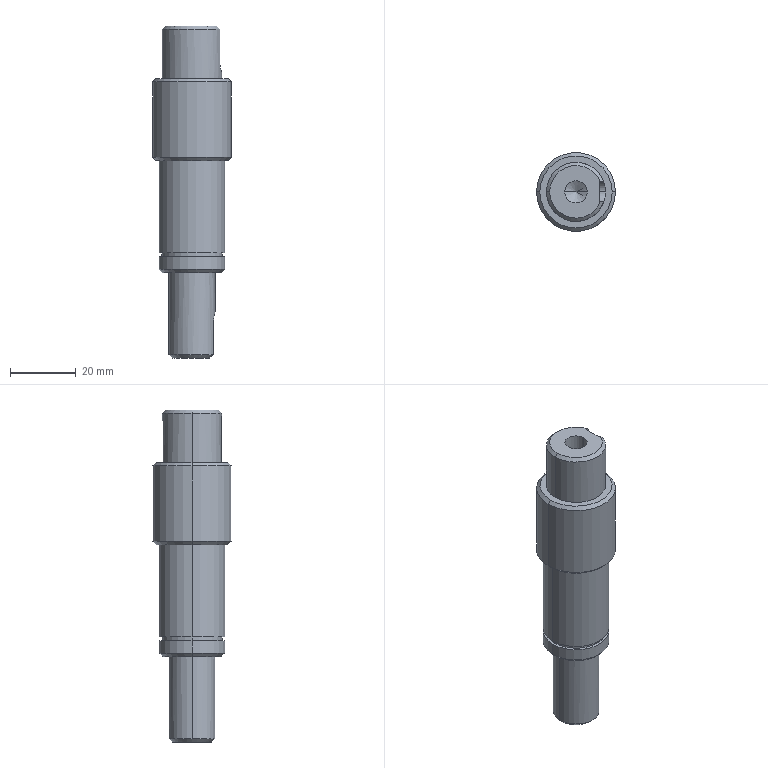Part | STEP file | Cut-off drive shaft | 1 solid | 42 faces | box 24 x 24 x 101 mm | volume 28813 mm3 | cylinder 18 | plane 13 | cone 11 | commonest cylinder face diameters 20 x4 5 x2 6 x2 6.8 x2 14 x2 18 x2
STEP:
#1=CARTESIAN_POINT('',(11.,0.,0.));
#2=VERTEX_POINT('',#1);
#3=CARTESIAN_POINT('',(-11.,0.,0.));
#4=VERTEX_POINT('',#3);
#5=CARTESIAN_POINT('',(0.,0.,0.));
#6=DIRECTION('',(0.,0.,1.));
#7=DIRECTION('',(-1.,0.,0.));
#8=AXIS2_PLACEMENT_3D('',#5,#6,#7);
#9=CIRCLE('',#8,11.);
#10=EDGE_CURVE('',#2,#4,#9,.T.);
#11=ORIENTED_EDGE('',*,*,#10,.F.);
#12=CARTESIAN_POINT('',(12.,0.,-1.));
#13=VERTEX_POINT('',#12);
#14=CARTESIAN_POINT('',(12.,0.,-1.));
#15=DIRECTION('',(0.7071,0.,-0.7071));
#16=VECTOR('',#15,1000.);
#17=LINE('',#14,#16);
#18=EDGE_CURVE('',#2,#13,#17,.T.);
#19=ORIENTED_EDGE('',*,*,#18,.T.);
#20=CARTESIAN_POINT('',(-12.,0.,-1.));
#21=VERTEX_POINT('',#20);
#22=CARTESIAN_POINT('',(0.,0.,-1.));
#23=DIRECTION('',(0.,0.,-1.));
#24=DIRECTION('',(-1.,0.,0.));
#25=AXIS2_PLACEMENT_3D('',#22,#23,#24);
#26=CIRCLE('',#25,12.);
#27=EDGE_CURVE('',#21,#13,#26,.T.);
#28=ORIENTED_EDGE('',*,*,#27,.F.);
#29=CARTESIAN_POINT('',(-12.,0.,-1.));
#30=DIRECTION('',(-0.7071,0.,-0.7071));
#31=VECTOR('',#30,1000.);
#32=LINE('',#29,#31);
#33=EDGE_CURVE('',#4,#21,#32,.T.);
#34=ORIENTED_EDGE('',*,*,#33,.F.);
#35=EDGE_LOOP('',(#11,#19,#28,#34));
#36=FACE_OUTER_BOUND('',#35,.T.);
#37=CARTESIAN_POINT('',(0.,0.,-1.));
#38=DIRECTION('',(0.,0.,-1.));
#39=DIRECTION('',(-1.,0.,0.));
#40=AXIS2_PLACEMENT_3D('',#37,#38,#39);
#41=CONICAL_SURFACE('',#40,12.,0.7854);
#42=ADVANCED_FACE('',(#36),#41,.T.);
#43=CARTESIAN_POINT('',(-11.,0.,-25.));
#44=VERTEX_POINT('',#43);
#45=CARTESIAN_POINT('',(11.,0.,-25.));
#46=VERTEX_POINT('',#45);
#47=CARTESIAN_POINT('',(0.,0.,-25.));
#48=DIRECTION('',(0.,0.,-1.));
#49=DIRECTION('',(-1.,0.,0.));
#50=AXIS2_PLACEMENT_3D('',#47,#48,#49);
#51=CIRCLE('',#50,11.);
#52=EDGE_CURVE('',#44,#46,#51,.T.);
#53=ORIENTED_EDGE('',*,*,#52,.F.);
#54=CARTESIAN_POINT('',(-12.,0.,-24.));
#55=VERTEX_POINT('',#54);
#56=CARTESIAN_POINT('',(-11.,0.,-25.));
#57=DIRECTION('',(-0.7071,0.,0.7071));
#58=VECTOR('',#57,1000.);
#59=LINE('',#56,#58);
#60=EDGE_CURVE('',#44,#55,#59,.T.);
#61=ORIENTED_EDGE('',*,*,#60,.T.);
#62=CARTESIAN_POINT('',(12.,0.,-24.));
#63=VERTEX_POINT('',#62);
#64=CARTESIAN_POINT('',(0.,0.,-24.));
#65=DIRECTION('',(0.,0.,1.));
#66=DIRECTION('',(-1.,0.,0.));
#67=AXIS2_PLACEMENT_3D('',#64,#65,#66);
#68=CIRCLE('',#67,12.);
#69=EDGE_CURVE('',#63,#55,#68,.T.);
#70=ORIENTED_EDGE('',*,*,#69,.F.);
#71=CARTESIAN_POINT('',(11.,0.,-25.));
#72=DIRECTION('',(0.7071,0.,0.7071));
#73=VECTOR('',#72,1000.);
#74=LINE('',#71,#73);
#75=EDGE_CURVE('',#46,#63,#74,.T.);
#76=ORIENTED_EDGE('',*,*,#75,.F.);
#77=EDGE_LOOP('',(#53,#61,#70,#76));
#78=FACE_OUTER_BOUND('',#77,.T.);
#79=CARTESIAN_POINT('',(0.,0.,-25.));
#80=DIRECTION('',(0.,0.,1.));
#81=DIRECTION('',(1.,0.,0.));
#82=AXIS2_PLACEMENT_3D('',#79,#80,#81);
#83=CONICAL_SURFACE('',#82,11.,0.7854);
#84=ADVANCED_FACE('',(#78),#83,.T.);
#85=CARTESIAN_POINT('',(-9.,0.,-59.));
#86=VERTEX_POINT('',#85);
#87=CARTESIAN_POINT('',(9.,0.,-59.));
#88=VERTEX_POINT('',#87);
#89=CARTESIAN_POINT('',(0.,0.,-59.));
#90=DIRECTION('',(0.,0.,-1.));
#91=DIRECTION('',(-1.,0.,0.));
#92=AXIS2_PLACEMENT_3D('',#89,#90,#91);
#93=CIRCLE('',#92,9.);
#94=EDGE_CURVE('',#86,#88,#93,.T.);
#95=ORIENTED_EDGE('',*,*,#94,.F.);
#96=CARTESIAN_POINT('',(-10.,0.,-58.));
#97=VERTEX_POINT('',#96);
#98=CARTESIAN_POINT('',(-9.,0.,-59.));
#99=DIRECTION('',(-0.7071,0.,0.7071));
#100=VECTOR('',#99,1000.);
#101=LINE('',#98,#100);
#102=EDGE_CURVE('',#86,#97,#101,.T.);
#103=ORIENTED_EDGE('',*,*,#102,.T.);
#104=CARTESIAN_POINT('',(10.,0.,-58.));
#105=VERTEX_POINT('',#104);
#106=CARTESIAN_POINT('',(0.,0.,-58.));
#107=DIRECTION('',(0.,0.,1.));
#108=DIRECTION('',(-1.,0.,0.));
#109=AXIS2_PLACEMENT_3D('',#106,#107,#108);
#110=CIRCLE('',#109,10.);
#111=EDGE_CURVE('',#105,#97,#110,.T.);
#112=ORIENTED_EDGE('',*,*,#111,.F.);
#113=CARTESIAN_POINT('',(9.,0.,-59.));
#114=DIRECTION('',(0.7071,0.,0.7071));
#115=VECTOR('',#114,1000.);
#116=LINE('',#113,#115);
#117=EDGE_CURVE('',#88,#105,#116,.T.);
#118=ORIENTED_EDGE('',*,*,#117,.F.);
#119=EDGE_LOOP('',(#95,#103,#112,#118));
#120=FACE_OUTER_BOUND('',#119,.T.);
#121=CARTESIAN_POINT('',(0.,0.,-59.));
#122=DIRECTION('',(0.,0.,1.));
#123=DIRECTION('',(1.,0.,0.));
#124=AXIS2_PLACEMENT_3D('',#121,#122,#123);
#125=CONICAL_SURFACE('',#124,9.,0.7854);
#126=ADVANCED_FACE('',(#120),#125,.T.);
#127=CARTESIAN_POINT('',(-3.4,0.,-3.75));
#128=VERTEX_POINT('',#127);
#129=CARTESIAN_POINT('',(3.4,0.,-3.75));
#130=VERTEX_POINT('',#129);
#131=CARTESIAN_POINT('',(0.,0.,-3.75));
#132=DIRECTION('',(0.,0.,1.));
#133=DIRECTION('',(1.,0.,0.));
#134=AXIS2_PLACEMENT_3D('',#131,#132,#133);
#135=CIRCLE('',#134,3.4);
#136=EDGE_CURVE('',#128,#130,#135,.T.);
#137=ORIENTED_EDGE('',*,*,#136,.F.);
#138=CARTESIAN_POINT('',(-3.4,0.,16.));
#139=VERTEX_POINT('',#138);
#140=CARTESIAN_POINT('',(-3.4,0.,16.));
#141=DIRECTION('',(0.,0.,1.));
#142=VECTOR('',#141,1000.);
#143=LINE('',#140,#142);
#144=EDGE_CURVE('',#128,#139,#143,.T.);
#145=ORIENTED_EDGE('',*,*,#144,.T.);
#146=CARTESIAN_POINT('',(3.4,0.,16.));
#147=VERTEX_POINT('',#146);
#148=CARTESIAN_POINT('',(0.,0.,16.));
#149=DIRECTION('',(0.,0.,1.));
#150=DIRECTION('',(1.,0.,0.));
#151=AXIS2_PLACEMENT_3D('',#148,#149,#150);
#152=CIRCLE('',#151,3.4);
#153=EDGE_CURVE('',#139,#147,#152,.T.);
#154=ORIENTED_EDGE('',*,*,#153,.T.);
#155=CARTESIAN_POINT('',(3.4,0.,16.));
#156=DIRECTION('',(0.,0.,1.));
#157=VECTOR('',#156,1000.);
#158=LINE('',#155,#157);
#159=EDGE_CURVE('',#130,#147,#158,.T.);
#160=ORIENTED_EDGE('',*,*,#159,.F.);
#161=EDGE_LOOP('',(#137,#145,#154,#160));
#162=FACE_OUTER_BOUND('',#161,.T.);
#163=CARTESIAN_POINT('',(0.,0.,16.));
#164=DIRECTION('',(0.,0.,1.));
#165=DIRECTION('',(1.,0.,0.));
#166=AXIS2_PLACEMENT_3D('',#163,#164,#165);
#167=CYLINDRICAL_SURFACE('',#166,3.4);
#168=ADVANCED_FACE('',(#162),#167,.F.);
#169=CARTESIAN_POINT('',(0.,0.,-5.793));
#170=VERTEX_POINT('',#169);
#171=CARTESIAN_POINT('',(3.4,0.,-3.75));
#172=DIRECTION('',(0.8572,0.,0.515));
#173=VECTOR('',#172,1000.);
#174=LINE('',#171,#173);
#175=EDGE_CURVE('',#170,#130,#174,.T.);
#176=ORIENTED_EDGE('',*,*,#175,.F.);
#177=CARTESIAN_POINT('',(-3.4,0.,-3.75));
#178=DIRECTION('',(-0.8572,0.,0.515));
#179=VECTOR('',#178,1000.);
#180=LINE('',#177,#179);
#181=EDGE_CURVE('',#170,#128,#180,.T.);
#182=ORIENTED_EDGE('',*,*,#181,.T.);
#183=ORIENTED_EDGE('',*,*,#136,.T.);
#184=EDGE_LOOP('',(#176,#182,#183));
#185=FACE_OUTER_BOUND('',#184,.T.);
#186=CARTESIAN_POINT('',(0.,0.,-3.75));
#187=DIRECTION('',(0.,0.,1.));
#188=DIRECTION('',(1.,0.,0.));
#189=AXIS2_PLACEMENT_3D('',#186,#187,#188);
#190=CONICAL_SURFACE('',#189,3.4,1.03);
#191=ADVANCED_FACE('',(#185),#190,.F.);
#192=CARTESIAN_POINT('',(6.538,2.5,-84.));
#193=VERTEX_POINT('',#192);
#194=CARTESIAN_POINT('',(-7.,0.,-84.));
#195=VERTEX_POINT('',#194);
#196=CARTESIAN_POINT('',(0.,0.,-84.));
#197=DIRECTION('',(0.,0.,1.));
#198=DIRECTION('',(-1.,0.,0.));
#199=AXIS2_PLACEMENT_3D('',#196,#197,#198);
#200=CIRCLE('',#199,7.);
#201=EDGE_CURVE('',#193,#195,#200,.T.);
#202=ORIENTED_EDGE('',*,*,#201,.T.);
#203=CARTESIAN_POINT('',(-7.,0.,-59.));
#204=VERTEX_POINT('',#203);
#205=CARTESIAN_POINT('',(-7.,0.,-85.));
#206=DIRECTION('',(0.,0.,1.));
#207=VECTOR('',#206,1000.);
#208=LINE('',#205,#207);
#209=EDGE_CURVE('',#195,#204,#208,.T.);
#210=ORIENTED_EDGE('',*,*,#209,.T.);
#211=CARTESIAN_POINT('',(7.,0.,-59.));
#212=VERTEX_POINT('',#211);
#213=CARTESIAN_POINT('',(0.,0.,-59.));
#214=DIRECTION('',(0.,0.,-1.));
#215=DIRECTION('',(-1.,0.,0.));
#216=AXIS2_PLACEMENT_3D('',#213,#214,#215);
#217=CIRCLE('',#216,7.);
#218=EDGE_CURVE('',#204,#212,#217,.T.);
#219=ORIENTED_EDGE('',*,*,#218,.T.);
#220=CARTESIAN_POINT('',(7.,0.,-71.));
#221=VERTEX_POINT('',#220);
#222=CARTESIAN_POINT('',(7.,0.,-85.));
#223=DIRECTION('',(0.,0.,1.));
#224=VECTOR('',#223,1000.);
#225=LINE('',#222,#224);
#226=EDGE_CURVE('',#221,#212,#225,.T.);
#227=ORIENTED_EDGE('',*,*,#226,.F.);
#228=CARTESIAN_POINT('',(6.538,2.5,-73.5));
#229=VERTEX_POINT('',#228);
#230=CARTESIAN_POINT('',(7.,0.,-71.));
#231=CARTESIAN_POINT('',(7.,0.1666,-71.));
#232=CARTESIAN_POINT('',(6.994,0.3301,-71.016));
#233=CARTESIAN_POINT('',(6.971,0.6514,-71.081));
#234=CARTESIAN_POINT('',(6.955,0.8108,-71.129));
#235=CARTESIAN_POINT('',(6.913,1.113,-71.255));
#236=CARTESIAN_POINT('',(6.888,1.256,-71.332));
#237=CARTESIAN_POINT('',(6.833,1.527,-71.514));
#238=CARTESIAN_POINT('',(6.803,1.654,-71.618));
#239=CARTESIAN_POINT('',(6.713,1.996,-71.961));
#240=CARTESIAN_POINT('',(6.653,2.182,-72.237));
#241=CARTESIAN_POINT('',(6.587,2.37,-72.687));
#242=CARTESIAN_POINT('',(6.569,2.418,-72.845));
#243=CARTESIAN_POINT('',(6.545,2.484,-73.169));
#244=CARTESIAN_POINT('',(6.538,2.5,-73.333));
#245=CARTESIAN_POINT('',(6.538,2.5,-73.5));
#246=B_SPLINE_CURVE_WITH_KNOTS('',3,(#230,#231,#232,#233,#234,#235,#236,#237,#238,#239,#240,#241,#242,#243,#244,#245),.UNSPECIFIED.,.F.,.F.,(4,2,2,2,2,2,2,4),(0.,0.0004923,0.0009846,0.001477,0.001969,0.002954,0.003446,0.003938),.UNSPECIFIED.);
#247=EDGE_CURVE('',#221,#229,#246,.T.);
#248=ORIENTED_EDGE('',*,*,#247,.T.);
#249=CARTESIAN_POINT('',(6.538,2.5,-85.));
#250=DIRECTION('',(0.,0.,-1.));
#251=VECTOR('',#250,1000.);
#252=LINE('',#249,#251);
#253=EDGE_CURVE('',#229,#193,#252,.T.);
#254=ORIENTED_EDGE('',*,*,#253,.T.);
#255=EDGE_LOOP('',(#202,#210,#219,#227,#248,#254));
#256=FACE_OUTER_BOUND('',#255,.T.);
#257=CARTESIAN_POINT('',(0.,0.,-85.));
#258=DIRECTION('',(0.,0.,1.));
#259=DIRECTION('',(1.,0.,0.));
#260=AXIS2_PLACEMENT_3D('',#257,#258,#259);
#261=CYLINDRICAL_SURFACE('',#260,7.);
#262=ADVANCED_FACE('',(#256),#261,.T.);
#263=ORIENTED_EDGE('',*,*,#111,.T.);
#264=CARTESIAN_POINT('',(-10.,0.,-54.2));
#265=VERTEX_POINT('',#264);
#266=CARTESIAN_POINT('',(-10.,0.,-55.));
#267=DIRECTION('',(0.,0.,1.));
#268=VECTOR('',#267,1000.);
#269=LINE('',#266,#268);
#270=EDGE_CURVE('',#97,#265,#269,.T.);
#271=ORIENTED_EDGE('',*,*,#270,.T.);
#272=CARTESIAN_POINT('',(10.,0.,-54.2));
#273=VERTEX_POINT('',#272);
#274=CARTESIAN_POINT('',(0.,0.,-54.2));
#275=DIRECTION('',(0.,0.,-1.));
#276=DIRECTION('',(-1.,0.,0.));
#277=AXIS2_PLACEMENT_3D('',#274,#275,#276);
#278=CIRCLE('',#277,10.);
#279=EDGE_CURVE('',#265,#273,#278,.T.);
#280=ORIENTED_EDGE('',*,*,#279,.T.);
#281=CARTESIAN_POINT('',(10.,0.,-55.));
#282=DIRECTION('',(0.,0.,1.));
#283=VECTOR('',#282,1000.);
#284=LINE('',#281,#283);
#285=EDGE_CURVE('',#105,#273,#284,.T.);
#286=ORIENTED_EDGE('',*,*,#285,.F.);
#287=EDGE_LOOP('',(#263,#271,#280,#286));
#288=FACE_OUTER_BOUND('',#287,.T.);
#289=CARTESIAN_POINT('',(0.,0.,-55.));
#290=DIRECTION('',(0.,0.,1.));
#291=DIRECTION('',(1.,0.,0.));
#292=AXIS2_PLACEMENT_3D('',#289,#290,#291);
#293=CYLINDRICAL_SURFACE('',#292,10.);
#294=ADVANCED_FACE('',(#288),#293,.T.);
#295=CARTESIAN_POINT('',(9.2,0.,-54.2));
#296=VERTEX_POINT('',#295);
#297=CARTESIAN_POINT('',(-9.2,0.,-54.2));
#298=VERTEX_POINT('',#297);
#299=CARTESIAN_POINT('',(0.,0.,-54.2));
#300=DIRECTION('',(0.,0.,1.));
#301=DIRECTION('',(1.,0.,0.));
#302=AXIS2_PLACEMENT_3D('',#299,#300,#301);
#303=CIRCLE('',#302,9.2);
#304=EDGE_CURVE('',#296,#298,#303,.T.);
#305=ORIENTED_EDGE('',*,*,#304,.T.);
#306=CARTESIAN_POINT('',(-9.2,0.,-53.));
#307=VERTEX_POINT('',#306);
#308=CARTESIAN_POINT('',(-9.2,0.,0.));
#309=DIRECTION('',(0.,0.,1.));
#310=VECTOR('',#309,1000.);
#311=LINE('',#308,#310);
#312=EDGE_CURVE('',#298,#307,#311,.T.);
#313=ORIENTED_EDGE('',*,*,#312,.T.);
#314=CARTESIAN_POINT('',(9.2,0.,-53.));
#315=VERTEX_POINT('',#314);
#316=CARTESIAN_POINT('',(0.,0.,-53.));
#317=DIRECTION('',(0.,0.,1.));
#318=DIRECTION('',(1.,0.,0.));
#319=AXIS2_PLACEMENT_3D('',#316,#317,#318);
#320=CIRCLE('',#319,9.2);
#321=EDGE_CURVE('',#315,#307,#320,.T.);
#322=ORIENTED_EDGE('',*,*,#321,.F.);
#323=CARTESIAN_POINT('',(9.2,0.,0.));
#324=DIRECTION('',(0.,0.,1.));
#325=VECTOR('',#324,1000.);
#326=LINE('',#323,#325);
#327=EDGE_CURVE('',#296,#315,#326,.T.);
#328=ORIENTED_EDGE('',*,*,#327,.F.);
#329=EDGE_LOOP('',(#305,#313,#322,#328));
#330=FACE_OUTER_BOUND('',#329,.T.);
#331=CARTESIAN_POINT('',(0.,0.,0.));
#332=DIRECTION('',(0.,0.,1.));
#333=DIRECTION('',(1.,0.,0.));
#334=AXIS2_PLACEMENT_3D('',#331,#332,#333);
#335=CYLINDRICAL_SURFACE('',#334,9.2);
#336=ADVANCED_FACE('',(#330),#335,.T.);
#337=CARTESIAN_POINT('',(10.,0.,-53.));
#338=VERTEX_POINT('',#337);
#339=CARTESIAN_POINT('',(-10.,0.,-53.));
#340=VERTEX_POINT('',#339);
#341=CARTESIAN_POINT('',(0.,0.,-53.));
#342=DIRECTION('',(0.,0.,1.));
#343=DIRECTION('',(1.,0.,0.));
#344=AXIS2_PLACEMENT_3D('',#341,#342,#343);
#345=CIRCLE('',#344,10.);
#346=EDGE_CURVE('',#338,#340,#345,.T.);
#347=ORIENTED_EDGE('',*,*,#346,.T.);
#348=CARTESIAN_POINT('',(-10.,0.,-25.));
#349=VERTEX_POINT('',#348);
#350=CARTESIAN_POINT('',(-10.,0.,-55.));
#351=DIRECTION('',(0.,0.,1.));
#352=VECTOR('',#351,1000.);
#353=LINE('',#350,#352);
#354=EDGE_CURVE('',#340,#349,#353,.T.);
#355=ORIENTED_EDGE('',*,*,#354,.T.);
#356=CARTESIAN_POINT('',(10.,0.,-25.));
#357=VERTEX_POINT('',#356);
#358=CARTESIAN_POINT('',(0.,0.,-25.));
#359=DIRECTION('',(0.,0.,-1.));
#360=DIRECTION('',(-1.,0.,0.));
#361=AXIS2_PLACEMENT_3D('',#358,#359,#360);
#362=CIRCLE('',#361,10.);
#363=EDGE_CURVE('',#349,#357,#362,.T.);
#364=ORIENTED_EDGE('',*,*,#363,.T.);
#365=CARTESIAN_POINT('',(10.,0.,-55.));
#366=DIRECTION('',(0.,0.,1.));
#367=VECTOR('',#366,1000.);
#368=LINE('',#365,#367);
#369=EDGE_CURVE('',#338,#357,#368,.T.);
#370=ORIENTED_EDGE('',*,*,#369,.F.);
#371=EDGE_LOOP('',(#347,#355,#364,#370));
#372=FACE_OUTER_BOUND('',#371,.T.);
#373=CARTESIAN_POINT('',(0.,0.,-55.));
#374=DIRECTION('',(0.,0.,1.));
#375=DIRECTION('',(1.,0.,0.));
#376=AXIS2_PLACEMENT_3D('',#373,#374,#375);
#377=CYLINDRICAL_SURFACE('',#376,10.);
#378=ADVANCED_FACE('',(#372),#377,.T.);
#379=ORIENTED_EDGE('',*,*,#69,.T.);
#380=CARTESIAN_POINT('',(-12.,0.,-25.));
#381=DIRECTION('',(0.,0.,1.));
#382=VECTOR('',#381,1000.);
#383=LINE('',#380,#382);
#384=EDGE_CURVE('',#55,#21,#383,.T.);
#385=ORIENTED_EDGE('',*,*,#384,.T.);
#386=ORIENTED_EDGE('',*,*,#27,.T.);
#387=CARTESIAN_POINT('',(12.,0.,-25.));
#388=DIRECTION('',(0.,0.,1.));
#389=VECTOR('',#388,1000.);
#390=LINE('',#387,#389);
#391=EDGE_CURVE('',#63,#13,#390,.T.);
#392=ORIENTED_EDGE('',*,*,#391,.F.);
#393=EDGE_LOOP('',(#379,#385,#386,#392));
#394=FACE_OUTER_BOUND('',#393,.T.);
#395=CARTESIAN_POINT('',(0.,0.,-25.));
#396=DIRECTION('',(0.,0.,1.));
#397=DIRECTION('',(1.,0.,0.));
#398=AXIS2_PLACEMENT_3D('',#395,#396,#397);
#399=CYLINDRICAL_SURFACE('',#398,12.);
#400=ADVANCED_FACE('',(#394),#399,.T.);
#401=CARTESIAN_POINT('',(-8.,0.,16.));
#402=VERTEX_POINT('',#401);
#403=CARTESIAN_POINT('',(7.416,-3.,16.));
#404=VERTEX_POINT('',#403);
#405=CARTESIAN_POINT('',(0.,0.,16.));
#406=DIRECTION('',(0.,0.,1.));
#407=DIRECTION('',(1.,0.,0.));
#408=AXIS2_PLACEMENT_3D('',#405,#406,#407);
#409=CIRCLE('',#408,8.);
#410=EDGE_CURVE('',#402,#404,#409,.T.);
#411=ORIENTED_EDGE('',*,*,#410,.F.);
#412=CARTESIAN_POINT('',(-9.,0.,15.));
#413=VERTEX_POINT('',#412);
#414=CARTESIAN_POINT('',(-8.,0.,16.));
#415=DIRECTION('',(-0.7071,0.,-0.7071));
#416=VECTOR('',#415,1000.);
#417=LINE('',#414,#416);
#418=EDGE_CURVE('',#402,#413,#417,.T.);
#419=ORIENTED_EDGE('',*,*,#418,.T.);
#420=CARTESIAN_POINT('',(8.485,-3.,15.));
#421=VERTEX_POINT('',#420);
#422=CARTESIAN_POINT('',(0.,0.,15.));
#423=DIRECTION('',(0.,0.,-1.));
#424=DIRECTION('',(1.,0.,0.));
#425=AXIS2_PLACEMENT_3D('',#422,#423,#424);
#426=CIRCLE('',#425,9.);
#427=EDGE_CURVE('',#421,#413,#426,.T.);
#428=ORIENTED_EDGE('',*,*,#427,.F.);
#429=CARTESIAN_POINT('',(8.485,-3.,15.));
#430=CARTESIAN_POINT('',(8.13,-3.,15.335));
#431=CARTESIAN_POINT('',(7.774,-3.,15.668));
#432=CARTESIAN_POINT('',(7.416,-3.,16.));
#433=B_SPLINE_CURVE_WITH_KNOTS('',3,(#429,#430,#431,#432),.UNSPECIFIED.,.F.,.F.,(4,4),(0.003025,0.004489),.UNSPECIFIED.);
#434=EDGE_CURVE('',#421,#404,#433,.T.);
#435=ORIENTED_EDGE('',*,*,#434,.T.);
#436=EDGE_LOOP('',(#411,#419,#428,#435));
#437=FACE_OUTER_BOUND('',#436,.T.);
#438=CARTESIAN_POINT('',(0.,0.,16.));
#439=DIRECTION('',(0.,0.,-1.));
#440=DIRECTION('',(-1.,0.,0.));
#441=AXIS2_PLACEMENT_3D('',#438,#439,#440);
#442=CONICAL_SURFACE('',#441,8.,0.7854);
#443=ADVANCED_FACE('',(#437),#442,.T.);
#444=CARTESIAN_POINT('',(8.485,3.,5.));
#445=VERTEX_POINT('',#444);
#446=CARTESIAN_POINT('',(9.,0.,2.));
#447=VERTEX_POINT('',#446);
#448=CARTESIAN_POINT('',(8.485,3.,5.));
#449=CARTESIAN_POINT('',(8.485,3.,4.8));
#450=CARTESIAN_POINT('',(8.492,2.98,4.604));
#451=CARTESIAN_POINT('',(8.519,2.903,4.219));
#452=CARTESIAN_POINT('',(8.539,2.845,4.028));
#453=CARTESIAN_POINT('',(8.588,2.694,3.666));
#454=CARTESIAN_POINT('',(8.616,2.602,3.494));
#455=CARTESIAN_POINT('',(8.679,2.385,3.169));
#456=CARTESIAN_POINT('',(8.713,2.259,3.017));
#457=CARTESIAN_POINT('',(8.813,1.848,2.605));
#458=CARTESIAN_POINT('',(8.879,1.516,2.382));
#459=CARTESIAN_POINT('',(8.949,0.9753,2.156));
#460=CARTESIAN_POINT('',(8.968,0.7852,2.098));
#461=CARTESIAN_POINT('',(8.993,0.3966,2.02));
#462=CARTESIAN_POINT('',(9.,0.1996,2.));
#463=CARTESIAN_POINT('',(9.,0.,2.));
#464=B_SPLINE_CURVE_WITH_KNOTS('',3,(#448,#449,#450,#451,#452,#453,#454,#455,#456,#457,#458,#459,#460,#461,#462,#463),.UNSPECIFIED.,.F.,.F.,(4,2,2,2,2,2,2,4),(0.,0.0005901,0.00118,0.00177,0.00236,0.00354,0.00413,0.004721),.UNSPECIFIED.);
#465=EDGE_CURVE('',#445,#447,#464,.T.);
#466=ORIENTED_EDGE('',*,*,#465,.T.);
#467=CARTESIAN_POINT('',(9.,0.,0.));
#468=VERTEX_POINT('',#467);
#469=CARTESIAN_POINT('',(9.,0.,16.));
#470=DIRECTION('',(0.,0.,-1.));
#471=VECTOR('',#470,1000.);
#472=LINE('',#469,#471);
#473=EDGE_CURVE('',#447,#468,#472,.T.);
#474=ORIENTED_EDGE('',*,*,#473,.T.);
#475=CARTESIAN_POINT('',(-9.,0.,0.));
#476=VERTEX_POINT('',#475);
#477=CARTESIAN_POINT('',(0.,0.,0.));
#478=DIRECTION('',(0.,0.,-1.));
#479=DIRECTION('',(-1.,0.,0.));
#480=AXIS2_PLACEMENT_3D('',#477,#478,#479);
#481=CIRCLE('',#480,9.);
#482=EDGE_CURVE('',#476,#468,#481,.T.);
#483=ORIENTED_EDGE('',*,*,#482,.F.);
#484=CARTESIAN_POINT('',(-9.,0.,16.));
#485=DIRECTION('',(0.,0.,-1.));
#486=VECTOR('',#485,1000.);
#487=LINE('',#484,#486);
#488=EDGE_CURVE('',#413,#476,#487,.T.);
#489=ORIENTED_EDGE('',*,*,#488,.F.);
#490=CARTESIAN_POINT('',(8.485,3.,15.));
#491=VERTEX_POINT('',#490);
#492=CARTESIAN_POINT('',(0.,0.,15.));
#493=DIRECTION('',(0.,0.,-1.));
#494=DIRECTION('',(1.,0.,0.));
#495=AXIS2_PLACEMENT_3D('',#492,#493,#494);
#496=CIRCLE('',#495,9.);
#497=EDGE_CURVE('',#413,#491,#496,.T.);
#498=ORIENTED_EDGE('',*,*,#497,.T.);
#499=CARTESIAN_POINT('',(8.485,3.,16.));
#500=DIRECTION('',(0.,0.,-1.));
#501=VECTOR('',#500,1000.);
#502=LINE('',#499,#501);
#503=EDGE_CURVE('',#491,#445,#502,.T.);
#504=ORIENTED_EDGE('',*,*,#503,.T.);
#505=EDGE_LOOP('',(#466,#474,#483,#489,#498,#504));
#506=FACE_OUTER_BOUND('',#505,.T.);
#507=CARTESIAN_POINT('',(0.,0.,16.));
#508=DIRECTION('',(0.,0.,-1.));
#509=DIRECTION('',(-1.,0.,0.));
#510=AXIS2_PLACEMENT_3D('',#507,#508,#509);
#511=CYLINDRICAL_SURFACE('',#510,9.);
#512=ADVANCED_FACE('',(#506),#511,.T.);
#513=ORIENTED_EDGE('',*,*,#473,.F.);
#514=CARTESIAN_POINT('',(8.485,-3.,5.));
#515=VERTEX_POINT('',#514);
#516=CARTESIAN_POINT('',(9.,0.,2.));
#517=CARTESIAN_POINT('',(9.,-0.1996,2.));
#518=CARTESIAN_POINT('',(8.993,-0.3957,2.02));
#519=CARTESIAN_POINT('',(8.968,-0.7809,2.097));
#520=CARTESIAN_POINT('',(8.949,-0.9721,2.155));
#521=CARTESIAN_POINT('',(8.902,-1.335,2.306));
#522=CARTESIAN_POINT('',(8.875,-1.506,2.398));
#523=CARTESIAN_POINT('',(8.813,-1.831,2.616));
#524=CARTESIAN_POINT('',(8.78,-1.984,2.741));
#525=CARTESIAN_POINT('',(8.68,-2.396,3.153));
#526=CARTESIAN_POINT('',(8.612,-2.618,3.485));
#527=CARTESIAN_POINT('',(8.539,-2.844,4.025));
#528=CARTESIAN_POINT('',(8.519,-2.902,4.215));
#529=CARTESIAN_POINT('',(8.492,-2.98,4.603));
#530=CARTESIAN_POINT('',(8.485,-3.,4.8));
#531=CARTESIAN_POINT('',(8.485,-3.,5.));
#532=B_SPLINE_CURVE_WITH_KNOTS('',3,(#516,#517,#518,#519,#520,#521,#522,#523,#524,#525,#526,#527,#528,#529,#530,#531),.UNSPECIFIED.,.F.,.F.,(4,2,2,2,2,2,2,4),(0.,0.0005901,0.00118,0.00177,0.00236,0.003541,0.004131,0.004721),.UNSPECIFIED.);
#533=EDGE_CURVE('',#447,#515,#532,.T.);
#534=ORIENTED_EDGE('',*,*,#533,.T.);
#535=CARTESIAN_POINT('',(8.485,-3.,16.));
#536=DIRECTION('',(0.,0.,-1.));
#537=VECTOR('',#536,1000.);
#538=LINE('',#535,#537);
#539=EDGE_CURVE('',#421,#515,#538,.T.);
#540=ORIENTED_EDGE('',*,*,#539,.F.);
#541=ORIENTED_EDGE('',*,*,#427,.T.);
#542=ORIENTED_EDGE('',*,*,#488,.T.);
#543=CARTESIAN_POINT('',(0.,0.,0.));
#544=DIRECTION('',(0.,0.,-1.));
#545=DIRECTION('',(-1.,0.,0.));
#546=AXIS2_PLACEMENT_3D('',#543,#544,#545);
#547=CIRCLE('',#546,9.);
#548=EDGE_CURVE('',#468,#476,#547,.T.);
#549=ORIENTED_EDGE('',*,*,#548,.F.);
#550=EDGE_LOOP('',(#513,#534,#540,#541,#542,#549));
#551=FACE_OUTER_BOUND('',#550,.T.);
#552=CARTESIAN_POINT('',(0.,0.,16.));
#553=DIRECTION('',(0.,0.,-1.));
#554=DIRECTION('',(-1.,0.,0.));
#555=AXIS2_PLACEMENT_3D('',#552,#553,#554);
#556=CYLINDRICAL_SURFACE('',#555,9.);
#557=ADVANCED_FACE('',(#551),#556,.T.);
#558=CARTESIAN_POINT('',(0.,0.,16.));
#559=DIRECTION('',(0.,0.,1.));
#560=DIRECTION('',(1.,0.,0.));
#561=AXIS2_PLACEMENT_3D('',#558,#559,#560);
#562=CIRCLE('',#561,3.4);
#563=EDGE_CURVE('',#147,#139,#562,.T.);
#564=ORIENTED_EDGE('',*,*,#563,.F.);
#565=ORIENTED_EDGE('',*,*,#153,.F.);
#566=EDGE_LOOP('',(#564,#565));
#567=FACE_BOUND('',#566,.T.);
#568=CARTESIAN_POINT('',(7.416,3.,16.));
#569=VERTEX_POINT('',#568);
#570=CARTESIAN_POINT('',(0.,0.,16.));
#571=DIRECTION('',(0.,0.,1.));
#572=DIRECTION('',(1.,0.,0.));
#573=AXIS2_PLACEMENT_3D('',#570,#571,#572);
#574=CIRCLE('',#573,8.);
#575=EDGE_CURVE('',#569,#402,#574,.T.);
#576=ORIENTED_EDGE('',*,*,#575,.T.);
#577=ORIENTED_EDGE('',*,*,#410,.T.);
#578=CARTESIAN_POINT('',(7.,-3.,16.));
#579=VERTEX_POINT('',#578);
#580=CARTESIAN_POINT('',(10.939,-3.,16.));
#581=DIRECTION('',(1.,0.,0.));
#582=VECTOR('',#581,1000.);
#583=LINE('',#580,#582);
#584=EDGE_CURVE('',#579,#404,#583,.T.);
#585=ORIENTED_EDGE('',*,*,#584,.F.);
#586=CARTESIAN_POINT('',(7.,3.,16.));
#587=VERTEX_POINT('',#586);
#588=CARTESIAN_POINT('',(7.,-3.,16.));
#589=DIRECTION('',(0.,1.,0.));
#590=VECTOR('',#589,1000.);
#591=LINE('',#588,#590);
#592=EDGE_CURVE('',#579,#587,#591,.T.);
#593=ORIENTED_EDGE('',*,*,#592,.T.);
#594=CARTESIAN_POINT('',(10.939,3.,16.));
#595=DIRECTION('',(1.,0.,0.));
#596=VECTOR('',#595,1000.);
#597=LINE('',#594,#596);
#598=EDGE_CURVE('',#587,#569,#597,.T.);
#599=ORIENTED_EDGE('',*,*,#598,.T.);
#600=EDGE_LOOP('',(#576,#577,#585,#593,#599));
#601=FACE_OUTER_BOUND('',#600,.T.);
#602=CARTESIAN_POINT('',(0.,0.,16.));
#603=DIRECTION('',(0.,0.,1.));
#604=DIRECTION('',(1.,0.,0.));
#605=AXIS2_PLACEMENT_3D('',#602,#603,#604);
#606=PLANE('',#605);
#607=ADVANCED_FACE('',(#567,#601),#606,.T.);
#608=ORIENTED_EDGE('',*,*,#418,.F.);
#609=ORIENTED_EDGE('',*,*,#575,.F.);
#610=CARTESIAN_POINT('',(8.485,3.,15.));
#611=CARTESIAN_POINT('',(8.13,3.,15.335));
#612=CARTESIAN_POINT('',(7.774,3.,15.668));
#613=CARTESIAN_POINT('',(7.416,3.,16.));
#614=B_SPLINE_CURVE_WITH_KNOTS('',3,(#610,#611,#612,#613),.UNSPECIFIED.,.F.,.F.,(4,4),(0.003025,0.004489),.UNSPECIFIED.);
#615=EDGE_CURVE('',#491,#569,#614,.T.);
#616=ORIENTED_EDGE('',*,*,#615,.F.);
#617=ORIENTED_EDGE('',*,*,#497,.F.);
#618=EDGE_LOOP('',(#608,#609,#616,#617));
#619=FACE_OUTER_BOUND('',#618,.T.);
#620=CARTESIAN_POINT('',(0.,0.,16.));
#621=DIRECTION('',(0.,0.,-1.));
#622=DIRECTION('',(-1.,0.,0.));
#623=AXIS2_PLACEMENT_3D('',#620,#621,#622);
#624=CONICAL_SURFACE('',#623,8.,0.7854);
#625=ADVANCED_FACE('',(#619),#624,.T.);
#626=ORIENTED_EDGE('',*,*,#384,.F.);
#627=CARTESIAN_POINT('',(0.,0.,-24.));
#628=DIRECTION('',(0.,0.,1.));
#629=DIRECTION('',(-1.,0.,0.));
#630=AXIS2_PLACEMENT_3D('',#627,#628,#629);
#631=CIRCLE('',#630,12.);
#632=EDGE_CURVE('',#55,#63,#631,.T.);
#633=ORIENTED_EDGE('',*,*,#632,.T.);
#634=ORIENTED_EDGE('',*,*,#391,.T.);
#635=CARTESIAN_POINT('',(0.,0.,-1.));
#636=DIRECTION('',(0.,0.,-1.));
#637=DIRECTION('',(-1.,0.,0.));
#638=AXIS2_PLACEMENT_3D('',#635,#636,#637);
#639=CIRCLE('',#638,12.);
#640=EDGE_CURVE('',#13,#21,#639,.T.);
#641=ORIENTED_EDGE('',*,*,#640,.T.);
#642=EDGE_LOOP('',(#626,#633,#634,#641));
#643=FACE_OUTER_BOUND('',#642,.T.);
#644=CARTESIAN_POINT('',(0.,0.,-25.));
#645=DIRECTION('',(0.,0.,1.));
#646=DIRECTION('',(1.,0.,0.));
#647=AXIS2_PLACEMENT_3D('',#644,#645,#646);
#648=CYLINDRICAL_SURFACE('',#647,12.);
#649=ADVANCED_FACE('',(#643),#648,.T.);
#650=CARTESIAN_POINT('',(0.,0.,-25.));
#651=DIRECTION('',(0.,0.,-1.));
#652=DIRECTION('',(-1.,0.,0.));
#653=AXIS2_PLACEMENT_3D('',#650,#651,#652);
#654=CIRCLE('',#653,11.);
#655=EDGE_CURVE('',#46,#44,#654,.T.);
#656=ORIENTED_EDGE('',*,*,#655,.T.);
#657=ORIENTED_EDGE('',*,*,#52,.T.);
#658=EDGE_LOOP('',(#656,#657));
#659=FACE_OUTER_BOUND('',#658,.T.);
#660=CARTESIAN_POINT('',(0.,0.,-25.));
#661=DIRECTION('',(0.,0.,-1.));
#662=DIRECTION('',(-1.,0.,0.));
#663=AXIS2_PLACEMENT_3D('',#660,#661,#662);
#664=CIRCLE('',#663,10.);
#665=EDGE_CURVE('',#357,#349,#664,.T.);
#666=ORIENTED_EDGE('',*,*,#665,.F.);
#667=ORIENTED_EDGE('',*,*,#363,.F.);
#668=EDGE_LOOP('',(#666,#667));
#669=FACE_BOUND('',#668,.T.);
#670=CARTESIAN_POINT('',(0.,0.,-25.));
#671=DIRECTION('',(0.,0.,-1.));
#672=DIRECTION('',(-1.,0.,0.));
#673=AXIS2_PLACEMENT_3D('',#670,#671,#672);
#674=PLANE('',#673);
#675=ADVANCED_FACE('',(#659,#669),#674,.T.);
#676=CARTESIAN_POINT('',(0.,0.,0.));
#677=DIRECTION('',(0.,0.,1.));
#678=DIRECTION('',(-1.,0.,0.));
#679=AXIS2_PLACEMENT_3D('',#676,#677,#678);
#680=CIRCLE('',#679,11.);
#681=EDGE_CURVE('',#4,#2,#680,.T.);
#682=ORIENTED_EDGE('',*,*,#681,.T.);
#683=ORIENTED_EDGE('',*,*,#10,.T.);
#684=EDGE_LOOP('',(#682,#683));
#685=FACE_OUTER_BOUND('',#684,.T.);
#686=ORIENTED_EDGE('',*,*,#482,.T.);
#687=ORIENTED_EDGE('',*,*,#548,.T.);
#688=EDGE_LOOP('',(#686,#687));
#689=FACE_BOUND('',#688,.T.);
#690=CARTESIAN_POINT('',(0.,0.,0.));
#691=DIRECTION('',(0.,0.,-1.));
#692=DIRECTION('',(-1.,0.,0.));
#693=AXIS2_PLACEMENT_3D('',#690,#691,#692);
#694=PLANE('',#693);
#695=ADVANCED_FACE('',(#685,#689),#694,.F.);
#696=ORIENTED_EDGE('',*,*,#354,.F.);
#697=CARTESIAN_POINT('',(0.,0.,-53.));
#698=DIRECTION('',(0.,0.,1.));
#699=DIRECTION('',(1.,0.,0.));
#700=AXIS2_PLACEMENT_3D('',#697,#698,#699);
#701=CIRCLE('',#700,10.);
#702=EDGE_CURVE('',#340,#338,#701,.T.);
#703=ORIENTED_EDGE('',*,*,#702,.T.);
#704=ORIENTED_EDGE('',*,*,#369,.T.);
#705=ORIENTED_EDGE('',*,*,#665,.T.);
#706=EDGE_LOOP('',(#696,#703,#704,#705));
#707=FACE_OUTER_BOUND('',#706,.T.);
#708=CARTESIAN_POINT('',(0.,0.,-55.));
#709=DIRECTION('',(0.,0.,1.));
#710=DIRECTION('',(1.,0.,0.));
#711=AXIS2_PLACEMENT_3D('',#708,#709,#710);
#712=CYLINDRICAL_SURFACE('',#711,10.);
#713=ADVANCED_FACE('',(#707),#712,.T.);
#714=ORIENTED_EDGE('',*,*,#304,.F.);
#715=CARTESIAN_POINT('',(0.,0.,-54.2));
#716=DIRECTION('',(0.,0.,1.));
#717=DIRECTION('',(1.,0.,0.));
#718=AXIS2_PLACEMENT_3D('',#715,#716,#717);
#719=CIRCLE('',#718,9.2);
#720=EDGE_CURVE('',#298,#296,#719,.T.);
#721=ORIENTED_EDGE('',*,*,#720,.F.);
#722=EDGE_LOOP('',(#714,#721));
#723=FACE_BOUND('',#722,.T.);
#724=CARTESIAN_POINT('',(0.,0.,-54.2));
#725=DIRECTION('',(0.,0.,-1.));
#726=DIRECTION('',(-1.,0.,0.));
#727=AXIS2_PLACEMENT_3D('',#724,#725,#726);
#728=CIRCLE('',#727,10.);
#729=EDGE_CURVE('',#273,#265,#728,.T.);
#730=ORIENTED_EDGE('',*,*,#729,.F.);
#731=ORIENTED_EDGE('',*,*,#279,.F.);
#732=EDGE_LOOP('',(#730,#731));
#733=FACE_OUTER_BOUND('',#732,.T.);
#734=CARTESIAN_POINT('',(15.077,0.,-54.2));
#735=DIRECTION('',(0.,0.,-1.));
#736=DIRECTION('',(-1.,0.,0.));
#737=AXIS2_PLACEMENT_3D('',#734,#735,#736);
#738=PLANE('',#737);
#739=ADVANCED_FACE('',(#723,#733),#738,.F.);
#740=ORIENTED_EDGE('',*,*,#321,.T.);
#741=CARTESIAN_POINT('',(0.,0.,-53.));
#742=DIRECTION('',(0.,0.,1.));
#743=DIRECTION('',(1.,0.,0.));
#744=AXIS2_PLACEMENT_3D('',#741,#742,#743);
#745=CIRCLE('',#744,9.2);
#746=EDGE_CURVE('',#307,#315,#745,.T.);
#747=ORIENTED_EDGE('',*,*,#746,.T.);
#748=EDGE_LOOP('',(#740,#747));
#749=FACE_BOUND('',#748,.T.);
#750=ORIENTED_EDGE('',*,*,#346,.F.);
#751=ORIENTED_EDGE('',*,*,#702,.F.);
#752=EDGE_LOOP('',(#750,#751));
#753=FACE_OUTER_BOUND('',#752,.T.);
#754=CARTESIAN_POINT('',(15.077,0.,-53.));
#755=DIRECTION('',(0.,0.,1.));
#756=DIRECTION('',(1.,0.,0.));
#757=AXIS2_PLACEMENT_3D('',#754,#755,#756);
#758=PLANE('',#757);
#759=ADVANCED_FACE('',(#749,#753),#758,.F.);
#760=ORIENTED_EDGE('',*,*,#312,.F.);
#761=ORIENTED_EDGE('',*,*,#720,.T.);
#762=ORIENTED_EDGE('',*,*,#327,.T.);
#763=ORIENTED_EDGE('',*,*,#746,.F.);
#764=EDGE_LOOP('',(#760,#761,#762,#763));
#765=FACE_OUTER_BOUND('',#764,.T.);
#766=CARTESIAN_POINT('',(0.,0.,0.));
#767=DIRECTION('',(0.,0.,1.));
#768=DIRECTION('',(1.,0.,0.));
#769=AXIS2_PLACEMENT_3D('',#766,#767,#768);
#770=CYLINDRICAL_SURFACE('',#769,9.2);
#771=ADVANCED_FACE('',(#765),#770,.T.);
#772=ORIENTED_EDGE('',*,*,#270,.F.);
#773=CARTESIAN_POINT('',(0.,0.,-58.));
#774=DIRECTION('',(0.,0.,1.));
#775=DIRECTION('',(-1.,0.,0.));
#776=AXIS2_PLACEMENT_3D('',#773,#774,#775);
#777=CIRCLE('',#776,10.);
#778=EDGE_CURVE('',#97,#105,#777,.T.);
#779=ORIENTED_EDGE('',*,*,#778,.T.);
#780=ORIENTED_EDGE('',*,*,#285,.T.);
#781=ORIENTED_EDGE('',*,*,#729,.T.);
#782=EDGE_LOOP('',(#772,#779,#780,#781));
#783=FACE_OUTER_BOUND('',#782,.T.);
#784=CARTESIAN_POINT('',(0.,0.,-55.));
#785=DIRECTION('',(0.,0.,1.));
#786=DIRECTION('',(1.,0.,0.));
#787=AXIS2_PLACEMENT_3D('',#784,#785,#786);
#788=CYLINDRICAL_SURFACE('',#787,10.);
#789=ADVANCED_FACE('',(#783),#788,.T.);
#790=CARTESIAN_POINT('',(0.,0.,-59.));
#791=DIRECTION('',(0.,0.,-1.));
#792=DIRECTION('',(-1.,0.,0.));
#793=AXIS2_PLACEMENT_3D('',#790,#791,#792);
#794=CIRCLE('',#793,9.);
#795=EDGE_CURVE('',#88,#86,#794,.T.);
#796=ORIENTED_EDGE('',*,*,#795,.T.);
#797=ORIENTED_EDGE('',*,*,#94,.T.);
#798=EDGE_LOOP('',(#796,#797));
#799=FACE_OUTER_BOUND('',#798,.T.);
#800=CARTESIAN_POINT('',(0.,0.,-59.));
#801=DIRECTION('',(0.,0.,-1.));
#802=DIRECTION('',(-1.,0.,0.));
#803=AXIS2_PLACEMENT_3D('',#800,#801,#802);
#804=CIRCLE('',#803,7.);
#805=EDGE_CURVE('',#212,#204,#804,.T.);
#806=ORIENTED_EDGE('',*,*,#805,.F.);
#807=ORIENTED_EDGE('',*,*,#218,.F.);
#808=EDGE_LOOP('',(#806,#807));
#809=FACE_BOUND('',#808,.T.);
#810=CARTESIAN_POINT('',(0.,0.,-59.));
#811=DIRECTION('',(0.,0.,-1.));
#812=DIRECTION('',(-1.,0.,0.));
#813=AXIS2_PLACEMENT_3D('',#810,#811,#812);
#814=PLANE('',#813);
#815=ADVANCED_FACE('',(#799,#809),#814,.T.);
#816=CARTESIAN_POINT('',(5.454,-2.5,-85.));
#817=VERTEX_POINT('',#816);
#818=CARTESIAN_POINT('',(4.5,-2.5,-85.));
#819=VERTEX_POINT('',#818);
#820=CARTESIAN_POINT('',(9.5,-2.5,-85.));
#821=DIRECTION('',(-1.,0.,0.));
#822=VECTOR('',#821,1000.);
#823=LINE('',#820,#822);
#824=EDGE_CURVE('',#817,#819,#823,.T.);
#825=ORIENTED_EDGE('',*,*,#824,.F.);
#826=CARTESIAN_POINT('',(5.454,2.5,-85.));
#827=VERTEX_POINT('',#826);
#828=CARTESIAN_POINT('',(0.,0.,-85.));
#829=DIRECTION('',(0.,0.,-1.));
#830=DIRECTION('',(-1.,0.,0.));
#831=AXIS2_PLACEMENT_3D('',#828,#829,#830);
#832=CIRCLE('',#831,6.);
#833=EDGE_CURVE('',#817,#827,#832,.T.);
#834=ORIENTED_EDGE('',*,*,#833,.T.);
#835=CARTESIAN_POINT('',(4.5,2.5,-85.));
#836=VERTEX_POINT('',#835);
#837=CARTESIAN_POINT('',(9.5,2.5,-85.));
#838=DIRECTION('',(1.,0.,0.));
#839=VECTOR('',#838,1000.);
#840=LINE('',#837,#839);
#841=EDGE_CURVE('',#836,#827,#840,.T.);
#842=ORIENTED_EDGE('',*,*,#841,.F.);
#843=CARTESIAN_POINT('',(4.5,-2.5,-85.));
#844=DIRECTION('',(0.,1.,0.));
#845=VECTOR('',#844,1000.);
#846=LINE('',#843,#845);
#847=EDGE_CURVE('',#819,#836,#846,.T.);
#848=ORIENTED_EDGE('',*,*,#847,.F.);
#849=EDGE_LOOP('',(#825,#834,#842,#848));
#850=FACE_OUTER_BOUND('',#849,.T.);
#851=CARTESIAN_POINT('',(0.,0.,-85.));
#852=DIRECTION('',(0.,0.,-1.));
#853=DIRECTION('',(-1.,0.,0.));
#854=AXIS2_PLACEMENT_3D('',#851,#852,#853);
#855=PLANE('',#854);
#856=ADVANCED_FACE('',(#850),#855,.T.);
#857=ORIENTED_EDGE('',*,*,#209,.F.);
#858=CARTESIAN_POINT('',(6.538,-2.5,-84.));
#859=VERTEX_POINT('',#858);
#860=CARTESIAN_POINT('',(0.,0.,-84.));
#861=DIRECTION('',(0.,0.,1.));
#862=DIRECTION('',(-1.,0.,0.));
#863=AXIS2_PLACEMENT_3D('',#860,#861,#862);
#864=CIRCLE('',#863,7.);
#865=EDGE_CURVE('',#195,#859,#864,.T.);
#866=ORIENTED_EDGE('',*,*,#865,.T.);
#867=CARTESIAN_POINT('',(6.538,-2.5,-73.5));
#868=VERTEX_POINT('',#867);
#869=CARTESIAN_POINT('',(6.538,-2.5,-85.));
#870=DIRECTION('',(0.,0.,1.));
#871=VECTOR('',#870,1000.);
#872=LINE('',#869,#871);
#873=EDGE_CURVE('',#859,#868,#872,.T.);
#874=ORIENTED_EDGE('',*,*,#873,.T.);
#875=CARTESIAN_POINT('',(6.538,-2.5,-73.5));
#876=CARTESIAN_POINT('',(6.538,-2.5,-73.333));
#877=CARTESIAN_POINT('',(6.545,-2.484,-73.17));
#878=CARTESIAN_POINT('',(6.569,-2.419,-72.849));
#879=CARTESIAN_POINT('',(6.587,-2.371,-72.689));
#880=CARTESIAN_POINT('',(6.631,-2.245,-72.388));
#881=CARTESIAN_POINT('',(6.656,-2.168,-72.245));
#882=CARTESIAN_POINT('',(6.713,-1.987,-71.974));
#883=CARTESIAN_POINT('',(6.743,-1.883,-71.847));
#884=CARTESIAN_POINT('',(6.833,-1.54,-71.504));
#885=CARTESIAN_POINT('',(6.892,-1.264,-71.319));
#886=CARTESIAN_POINT('',(6.954,-0.8135,-71.13));
#887=CARTESIAN_POINT('',(6.971,-0.6548,-71.082));
#888=CARTESIAN_POINT('',(6.994,-0.3308,-71.016));
#889=CARTESIAN_POINT('',(7.,-0.1666,-71.));
#890=CARTESIAN_POINT('',(7.,0.,-71.));
#891=B_SPLINE_CURVE_WITH_KNOTS('',3,(#875,#876,#877,#878,#879,#880,#881,#882,#883,#884,#885,#886,#887,#888,#889,#890),.UNSPECIFIED.,.F.,.F.,(4,2,2,2,2,2,2,4),(0.,0.0004923,0.0009846,0.001477,0.001969,0.002954,0.003446,0.003938),.UNSPECIFIED.);
#892=EDGE_CURVE('',#868,#221,#891,.T.);
#893=ORIENTED_EDGE('',*,*,#892,.T.);
#894=ORIENTED_EDGE('',*,*,#226,.T.);
#895=ORIENTED_EDGE('',*,*,#805,.T.);
#896=EDGE_LOOP('',(#857,#866,#874,#893,#894,#895));
#897=FACE_OUTER_BOUND('',#896,.T.);
#898=CARTESIAN_POINT('',(0.,0.,-85.));
#899=DIRECTION('',(0.,0.,1.));
#900=DIRECTION('',(1.,0.,0.));
#901=AXIS2_PLACEMENT_3D('',#898,#899,#900);
#902=CYLINDRICAL_SURFACE('',#901,7.);
#903=ADVANCED_FACE('',(#897),#902,.T.);
#904=ORIENTED_EDGE('',*,*,#181,.F.);
#905=ORIENTED_EDGE('',*,*,#175,.T.);
#906=CARTESIAN_POINT('',(0.,0.,-3.75));
#907=DIRECTION('',(0.,0.,1.));
#908=DIRECTION('',(1.,0.,0.));
#909=AXIS2_PLACEMENT_3D('',#906,#907,#908);
#910=CIRCLE('',#909,3.4);
#911=EDGE_CURVE('',#130,#128,#910,.T.);
#912=ORIENTED_EDGE('',*,*,#911,.T.);
#913=EDGE_LOOP('',(#904,#905,#912));
#914=FACE_OUTER_BOUND('',#913,.T.);
#915=CARTESIAN_POINT('',(0.,0.,-3.75));
#916=DIRECTION('',(0.,0.,1.));
#917=DIRECTION('',(1.,0.,0.));
#918=AXIS2_PLACEMENT_3D('',#915,#916,#917);
#919=CONICAL_SURFACE('',#918,3.4,1.03);
#920=ADVANCED_FACE('',(#914),#919,.F.);
#921=ORIENTED_EDGE('',*,*,#144,.F.);
#922=ORIENTED_EDGE('',*,*,#911,.F.);
#923=ORIENTED_EDGE('',*,*,#159,.T.);
#924=ORIENTED_EDGE('',*,*,#563,.T.);
#925=EDGE_LOOP('',(#921,#922,#923,#924));
#926=FACE_OUTER_BOUND('',#925,.T.);
#927=CARTESIAN_POINT('',(0.,0.,16.));
#928=DIRECTION('',(0.,0.,1.));
#929=DIRECTION('',(1.,0.,0.));
#930=AXIS2_PLACEMENT_3D('',#927,#928,#929);
#931=CYLINDRICAL_SURFACE('',#930,3.4);
#932=ADVANCED_FACE('',(#926),#931,.F.);
#933=ORIENTED_EDGE('',*,*,#539,.T.);
#934=CARTESIAN_POINT('',(7.,-3.,5.));
#935=VERTEX_POINT('',#934);
#936=CARTESIAN_POINT('',(0.,-3.,5.));
#937=DIRECTION('',(-1.,0.,0.));
#938=VECTOR('',#937,1000.);
#939=LINE('',#936,#938);
#940=EDGE_CURVE('',#515,#935,#939,.T.);
#941=ORIENTED_EDGE('',*,*,#940,.T.);
#942=CARTESIAN_POINT('',(7.,-3.,16.));
#943=DIRECTION('',(0.,0.,1.));
#944=VECTOR('',#943,1000.);
#945=LINE('',#942,#944);
#946=EDGE_CURVE('',#935,#579,#945,.T.);
#947=ORIENTED_EDGE('',*,*,#946,.T.);
#948=ORIENTED_EDGE('',*,*,#584,.T.);
#949=ORIENTED_EDGE('',*,*,#434,.F.);
#950=EDGE_LOOP('',(#933,#941,#947,#948,#949));
#951=FACE_OUTER_BOUND('',#950,.T.);
#952=CARTESIAN_POINT('',(0.,-3.,0.));
#953=DIRECTION('',(0.,1.,0.));
#954=DIRECTION('',(0.,0.,1.));
#955=AXIS2_PLACEMENT_3D('',#952,#953,#954);
#956=PLANE('',#955);
#957=ADVANCED_FACE('',(#951),#956,.T.);
#958=CARTESIAN_POINT('',(7.,3.,5.));
#959=VERTEX_POINT('',#958);
#960=CARTESIAN_POINT('',(7.,3.,16.));
#961=DIRECTION('',(0.,0.,1.));
#962=VECTOR('',#961,1000.);
#963=LINE('',#960,#962);
#964=EDGE_CURVE('',#959,#587,#963,.T.);
#965=ORIENTED_EDGE('',*,*,#964,.F.);
#966=CARTESIAN_POINT('',(8.485,3.,5.));
#967=DIRECTION('',(1.,0.,0.));
#968=VECTOR('',#967,1000.);
#969=LINE('',#966,#968);
#970=EDGE_CURVE('',#959,#445,#969,.T.);
#971=ORIENTED_EDGE('',*,*,#970,.T.);
#972=ORIENTED_EDGE('',*,*,#503,.F.);
#973=ORIENTED_EDGE('',*,*,#615,.T.);
#974=ORIENTED_EDGE('',*,*,#598,.F.);
#975=EDGE_LOOP('',(#965,#971,#972,#973,#974));
#976=FACE_OUTER_BOUND('',#975,.T.);
#977=CARTESIAN_POINT('',(0.,3.,0.));
#978=DIRECTION('',(0.,1.,0.));
#979=DIRECTION('',(0.,0.,1.));
#980=AXIS2_PLACEMENT_3D('',#977,#978,#979);
#981=PLANE('',#980);
#982=ADVANCED_FACE('',(#976),#981,.F.);
#983=ORIENTED_EDGE('',*,*,#946,.F.);
#984=CARTESIAN_POINT('',(7.,0.,2.));
#985=VERTEX_POINT('',#984);
#986=CARTESIAN_POINT('',(7.,0.,5.));
#987=DIRECTION('',(1.,0.,0.));
#988=DIRECTION('',(0.,0.,1.));
#989=AXIS2_PLACEMENT_3D('',#986,#987,#988);
#990=CIRCLE('',#989,3.);
#991=EDGE_CURVE('',#935,#985,#990,.T.);
#992=ORIENTED_EDGE('',*,*,#991,.T.);
#993=CARTESIAN_POINT('',(7.,0.,5.));
#994=DIRECTION('',(1.,0.,0.));
#995=DIRECTION('',(0.,0.,1.));
#996=AXIS2_PLACEMENT_3D('',#993,#994,#995);
#997=CIRCLE('',#996,3.);
#998=EDGE_CURVE('',#985,#959,#997,.T.);
#999=ORIENTED_EDGE('',*,*,#998,.T.);
#1000=ORIENTED_EDGE('',*,*,#964,.T.);
#1001=ORIENTED_EDGE('',*,*,#592,.F.);
#1002=EDGE_LOOP('',(#983,#992,#999,#1000,#1001));
#1003=FACE_OUTER_BOUND('',#1002,.T.);
#1004=CARTESIAN_POINT('',(7.,-3.,16.));
#1005=DIRECTION('',(-1.,0.,0.));
#1006=DIRECTION('',(0.,0.,1.));
#1007=AXIS2_PLACEMENT_3D('',#1004,#1005,#1006);
#1008=PLANE('',#1007);
#1009=ADVANCED_FACE('',(#1003),#1008,.F.);
#1010=CARTESIAN_POINT('',(7.,0.,2.));
#1011=DIRECTION('',(-1.,0.,0.));
#1012=VECTOR('',#1011,1000.);
#1013=LINE('',#1010,#1012);
#1014=EDGE_CURVE('',#447,#985,#1013,.T.);
#1015=ORIENTED_EDGE('',*,*,#1014,.F.);
#1016=ORIENTED_EDGE('',*,*,#465,.F.);
#1017=ORIENTED_EDGE('',*,*,#970,.F.);
#1018=ORIENTED_EDGE('',*,*,#998,.F.);
#1019=EDGE_LOOP('',(#1015,#1016,#1017,#1018));
#1020=FACE_OUTER_BOUND('',#1019,.T.);
#1021=CARTESIAN_POINT('',(10.939,0.,5.));
#1022=DIRECTION('',(1.,0.,0.));
#1023=DIRECTION('',(0.,0.,-1.));
#1024=AXIS2_PLACEMENT_3D('',#1021,#1022,#1023);
#1025=CYLINDRICAL_SURFACE('',#1024,3.);
#1026=ADVANCED_FACE('',(#1020),#1025,.F.);
#1027=ORIENTED_EDGE('',*,*,#533,.F.);
#1028=ORIENTED_EDGE('',*,*,#1014,.T.);
#1029=ORIENTED_EDGE('',*,*,#991,.F.);
#1030=ORIENTED_EDGE('',*,*,#940,.F.);
#1031=EDGE_LOOP('',(#1027,#1028,#1029,#1030));
#1032=FACE_OUTER_BOUND('',#1031,.T.);
#1033=CARTESIAN_POINT('',(0.,0.,5.));
#1034=DIRECTION('',(-1.,0.,0.));
#1035=DIRECTION('',(0.,0.,1.));
#1036=AXIS2_PLACEMENT_3D('',#1033,#1034,#1035);
#1037=CYLINDRICAL_SURFACE('',#1036,3.);
#1038=ADVANCED_FACE('',(#1032),#1037,.F.);
#1039=ORIENTED_EDGE('',*,*,#102,.F.);
#1040=ORIENTED_EDGE('',*,*,#795,.F.);
#1041=ORIENTED_EDGE('',*,*,#117,.T.);
#1042=ORIENTED_EDGE('',*,*,#778,.F.);
#1043=EDGE_LOOP('',(#1039,#1040,#1041,#1042));
#1044=FACE_OUTER_BOUND('',#1043,.T.);
#1045=CARTESIAN_POINT('',(0.,0.,-59.));
#1046=DIRECTION('',(0.,0.,1.));
#1047=DIRECTION('',(1.,0.,0.));
#1048=AXIS2_PLACEMENT_3D('',#1045,#1046,#1047);
#1049=CONICAL_SURFACE('',#1048,9.,0.7854);
#1050=ADVANCED_FACE('',(#1044),#1049,.T.);
#1051=ORIENTED_EDGE('',*,*,#60,.F.);
#1052=ORIENTED_EDGE('',*,*,#655,.F.);
#1053=ORIENTED_EDGE('',*,*,#75,.T.);
#1054=ORIENTED_EDGE('',*,*,#632,.F.);
#1055=EDGE_LOOP('',(#1051,#1052,#1053,#1054));
#1056=FACE_OUTER_BOUND('',#1055,.T.);
#1057=CARTESIAN_POINT('',(0.,0.,-25.));
#1058=DIRECTION('',(0.,0.,1.));
#1059=DIRECTION('',(1.,0.,0.));
#1060=AXIS2_PLACEMENT_3D('',#1057,#1058,#1059);
#1061=CONICAL_SURFACE('',#1060,11.,0.7854);
#1062=ADVANCED_FACE('',(#1056),#1061,.T.);
#1063=ORIENTED_EDGE('',*,*,#18,.F.);
#1064=ORIENTED_EDGE('',*,*,#681,.F.);
#1065=ORIENTED_EDGE('',*,*,#33,.T.);
#1066=ORIENTED_EDGE('',*,*,#640,.F.);
#1067=EDGE_LOOP('',(#1063,#1064,#1065,#1066));
#1068=FACE_OUTER_BOUND('',#1067,.T.);
#1069=CARTESIAN_POINT('',(0.,0.,-1.));
#1070=DIRECTION('',(0.,0.,-1.));
#1071=DIRECTION('',(-1.,0.,0.));
#1072=AXIS2_PLACEMENT_3D('',#1069,#1070,#1071);
#1073=CONICAL_SURFACE('',#1072,12.,0.7854);
#1074=ADVANCED_FACE('',(#1068),#1073,.T.);
#1075=ORIENTED_EDGE('',*,*,#873,.F.);
#1076=CARTESIAN_POINT('',(6.538,-2.5,-84.));
#1077=CARTESIAN_POINT('',(6.179,-2.5,-84.336));
#1078=CARTESIAN_POINT('',(5.818,-2.5,-84.669));
#1079=CARTESIAN_POINT('',(5.454,-2.5,-85.));
#1080=B_SPLINE_CURVE_WITH_KNOTS('',3,(#1076,#1077,#1078,#1079),.UNSPECIFIED.,.F.,.F.,(4,4),(0.,0.001475),.UNSPECIFIED.);
#1081=EDGE_CURVE('',#859,#817,#1080,.T.);
#1082=ORIENTED_EDGE('',*,*,#1081,.T.);
#1083=ORIENTED_EDGE('',*,*,#824,.T.);
#1084=CARTESIAN_POINT('',(4.5,-2.5,-73.5));
#1085=VERTEX_POINT('',#1084);
#1086=CARTESIAN_POINT('',(4.5,-2.5,-71.));
#1087=DIRECTION('',(0.,0.,-1.));
#1088=VECTOR('',#1087,1000.);
#1089=LINE('',#1086,#1088);
#1090=EDGE_CURVE('',#1085,#819,#1089,.T.);
#1091=ORIENTED_EDGE('',*,*,#1090,.F.);
#1092=CARTESIAN_POINT('',(6.538,-2.5,-73.5));
#1093=DIRECTION('',(1.,0.,0.));
#1094=VECTOR('',#1093,1000.);
#1095=LINE('',#1092,#1094);
#1096=EDGE_CURVE('',#1085,#868,#1095,.T.);
#1097=ORIENTED_EDGE('',*,*,#1096,.T.);
#1098=EDGE_LOOP('',(#1075,#1082,#1083,#1091,#1097));
#1099=FACE_OUTER_BOUND('',#1098,.T.);
#1100=CARTESIAN_POINT('',(9.5,-2.5,-71.));
#1101=DIRECTION('',(0.,-1.,0.));
#1102=DIRECTION('',(0.,0.,-1.));
#1103=AXIS2_PLACEMENT_3D('',#1100,#1101,#1102);
#1104=PLANE('',#1103);
#1105=ADVANCED_FACE('',(#1099),#1104,.F.);
#1106=ORIENTED_EDGE('',*,*,#841,.T.);
#1107=CARTESIAN_POINT('',(5.454,2.5,-85.));
#1108=CARTESIAN_POINT('',(5.818,2.5,-84.669));
#1109=CARTESIAN_POINT('',(6.179,2.5,-84.336));
#1110=CARTESIAN_POINT('',(6.538,2.5,-84.));
#1111=B_SPLINE_CURVE_WITH_KNOTS('',3,(#1107,#1108,#1109,#1110),.UNSPECIFIED.,.F.,.F.,(4,4),(0.,0.001475),.UNSPECIFIED.);
#1112=EDGE_CURVE('',#827,#193,#1111,.T.);
#1113=ORIENTED_EDGE('',*,*,#1112,.T.);
#1114=ORIENTED_EDGE('',*,*,#253,.F.);
#1115=CARTESIAN_POINT('',(4.5,2.5,-73.5));
#1116=VERTEX_POINT('',#1115);
#1117=CARTESIAN_POINT('',(4.5,2.5,-73.5));
#1118=DIRECTION('',(-1.,0.,0.));
#1119=VECTOR('',#1118,1000.);
#1120=LINE('',#1117,#1119);
#1121=EDGE_CURVE('',#229,#1116,#1120,.T.);
#1122=ORIENTED_EDGE('',*,*,#1121,.T.);
#1123=CARTESIAN_POINT('',(4.5,2.5,-71.));
#1124=DIRECTION('',(0.,0.,-1.));
#1125=VECTOR('',#1124,1000.);
#1126=LINE('',#1123,#1125);
#1127=EDGE_CURVE('',#1116,#836,#1126,.T.);
#1128=ORIENTED_EDGE('',*,*,#1127,.T.);
#1129=EDGE_LOOP('',(#1106,#1113,#1114,#1122,#1128));
#1130=FACE_OUTER_BOUND('',#1129,.T.);
#1131=CARTESIAN_POINT('',(9.5,2.5,-71.));
#1132=DIRECTION('',(0.,1.,0.));
#1133=DIRECTION('',(-1.,0.,0.));
#1134=AXIS2_PLACEMENT_3D('',#1131,#1132,#1133);
#1135=PLANE('',#1134);
#1136=ADVANCED_FACE('',(#1130),#1135,.F.);
#1137=ORIENTED_EDGE('',*,*,#1127,.F.);
#1138=CARTESIAN_POINT('',(4.5,0.,-71.));
#1139=VERTEX_POINT('',#1138);
#1140=CARTESIAN_POINT('',(4.5,0.,-73.5));
#1141=DIRECTION('',(1.,0.,0.));
#1142=DIRECTION('',(0.,-1.,0.));
#1143=AXIS2_PLACEMENT_3D('',#1140,#1141,#1142);
#1144=CIRCLE('',#1143,2.5);
#1145=EDGE_CURVE('',#1116,#1139,#1144,.T.);
#1146=ORIENTED_EDGE('',*,*,#1145,.T.);
#1147=CARTESIAN_POINT('',(4.5,0.,-73.5));
#1148=DIRECTION('',(1.,0.,0.));
#1149=DIRECTION('',(0.,-1.,0.));
#1150=AXIS2_PLACEMENT_3D('',#1147,#1148,#1149);
#1151=CIRCLE('',#1150,2.5);
#1152=EDGE_CURVE('',#1139,#1085,#1151,.T.);
#1153=ORIENTED_EDGE('',*,*,#1152,.T.);
#1154=ORIENTED_EDGE('',*,*,#1090,.T.);
#1155=ORIENTED_EDGE('',*,*,#847,.T.);
#1156=EDGE_LOOP('',(#1137,#1146,#1153,#1154,#1155));
#1157=FACE_OUTER_BOUND('',#1156,.T.);
#1158=CARTESIAN_POINT('',(4.5,-2.5,-71.));
#1159=DIRECTION('',(-1.,0.,0.));
#1160=DIRECTION('',(0.,-1.,0.));
#1161=AXIS2_PLACEMENT_3D('',#1158,#1159,#1160);
#1162=PLANE('',#1161);
#1163=ADVANCED_FACE('',(#1157),#1162,.F.);
#1164=ORIENTED_EDGE('',*,*,#1096,.F.);
#1165=ORIENTED_EDGE('',*,*,#1152,.F.);
#1166=CARTESIAN_POINT('',(4.5,0.,-71.));
#1167=DIRECTION('',(-1.,0.,0.));
#1168=VECTOR('',#1167,1000.);
#1169=LINE('',#1166,#1168);
#1170=EDGE_CURVE('',#221,#1139,#1169,.T.);
#1171=ORIENTED_EDGE('',*,*,#1170,.F.);
#1172=ORIENTED_EDGE('',*,*,#892,.F.);
#1173=EDGE_LOOP('',(#1164,#1165,#1171,#1172));
#1174=FACE_OUTER_BOUND('',#1173,.T.);
#1175=CARTESIAN_POINT('',(0.,0.,-73.5));
#1176=DIRECTION('',(1.,0.,0.));
#1177=DIRECTION('',(0.,0.,-1.));
#1178=AXIS2_PLACEMENT_3D('',#1175,#1176,#1177);
#1179=CYLINDRICAL_SURFACE('',#1178,2.5);
#1180=ADVANCED_FACE('',(#1174),#1179,.F.);
#1181=ORIENTED_EDGE('',*,*,#1145,.F.);
#1182=ORIENTED_EDGE('',*,*,#1121,.F.);
#1183=ORIENTED_EDGE('',*,*,#247,.F.);
#1184=ORIENTED_EDGE('',*,*,#1170,.T.);
#1185=EDGE_LOOP('',(#1181,#1182,#1183,#1184));
#1186=FACE_OUTER_BOUND('',#1185,.T.);
#1187=CARTESIAN_POINT('',(0.,0.,-73.5));
#1188=DIRECTION('',(-1.,0.,0.));
#1189=DIRECTION('',(0.,-1.,0.));
#1190=AXIS2_PLACEMENT_3D('',#1187,#1188,#1189);
#1191=CYLINDRICAL_SURFACE('',#1190,2.5);
#1192=ADVANCED_FACE('',(#1186),#1191,.F.);
#1193=ORIENTED_EDGE('',*,*,#1081,.F.);
#1194=ORIENTED_EDGE('',*,*,#865,.F.);
#1195=ORIENTED_EDGE('',*,*,#201,.F.);
#1196=ORIENTED_EDGE('',*,*,#1112,.F.);
#1197=ORIENTED_EDGE('',*,*,#833,.F.);
#1198=EDGE_LOOP('',(#1193,#1194,#1195,#1196,#1197));
#1199=FACE_OUTER_BOUND('',#1198,.T.);
#1200=CARTESIAN_POINT('',(0.,0.,-85.));
#1201=DIRECTION('',(0.,0.,1.));
#1202=DIRECTION('',(1.,0.,0.));
#1203=AXIS2_PLACEMENT_3D('',#1200,#1201,#1202);
#1204=CONICAL_SURFACE('',#1203,6.,0.7854);
#1205=ADVANCED_FACE('',(#1199),#1204,.T.);
#1206=CLOSED_SHELL('',(#42,#84,#126,#168,#191,#262,#294,#336,#378,#400,#443,#512,#557,#607,#625,#649,#675,#695,#713,#739,#759,#771,#789,#815,#856,#903,#920,#932,#957,#982,#1009,#1026,#1038,#1050,#1062,#1074,#1105,#1136,#1163,#1180,#1192,#1205));
#1207=MANIFOLD_SOLID_BREP('',#1206);
#1208=CARTESIAN_POINT('',(0.,0.,0.));
#1209=DIRECTION('',(0.,0.,1.));
#1210=DIRECTION('',(1.,0.,0.));
#1211=AXIS2_PLACEMENT_3D('',#1208,#1209,#1210);
#1212=(LENGTH_UNIT()NAMED_UNIT(*)SI_UNIT(.MILLI.,.METRE.));
#1213=UNCERTAINTY_MEASURE_WITH_UNIT(LENGTH_MEASURE(0.00001),#1212,'','');
#1214=(NAMED_UNIT(*)PLANE_ANGLE_UNIT()SI_UNIT($,.RADIAN.));
#1215=(NAMED_UNIT(*)SI_UNIT($,.STERADIAN.)SOLID_ANGLE_UNIT());
#1216=(GEOMETRIC_REPRESENTATION_CONTEXT(3)GLOBAL_UNCERTAINTY_ASSIGNED_CONTEXT((#1213))GLOBAL_UNIT_ASSIGNED_CONTEXT((#1212,#1214,#1215))REPRESENTATION_CONTEXT('',''));
#1217=ADVANCED_BREP_SHAPE_REPRESENTATION('',(#1207,#1211),#1216);